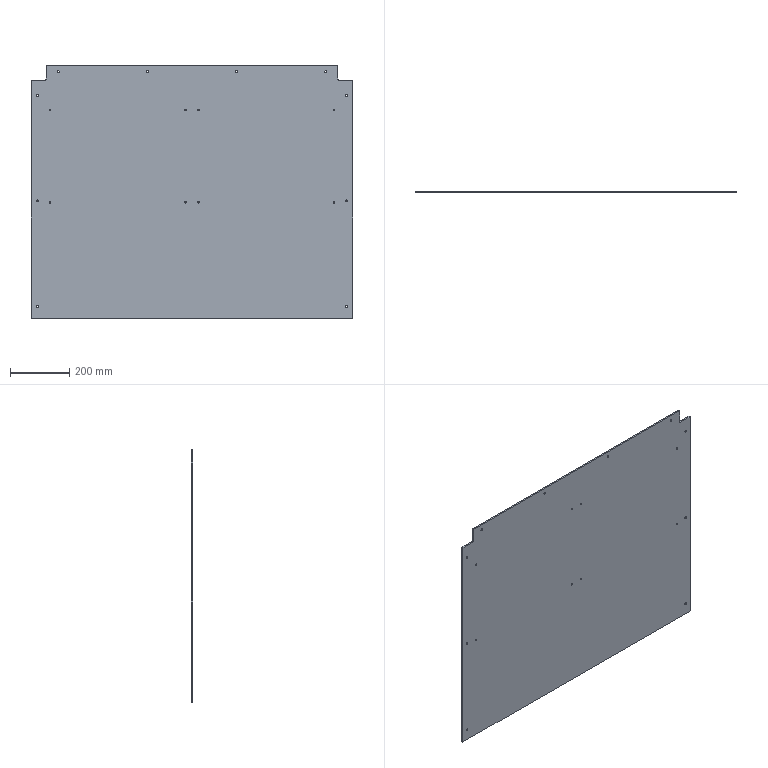Part | SolidWorks | features BaseBody 1 | 1 solid | 68 faces | box 1080 x 5 x 850 mm | volume 4561249 mm3 | cylinder 38 | cone 20 | plane 10 | commonest cylinder face diameters 6.6 x20 5 x16 10 x2